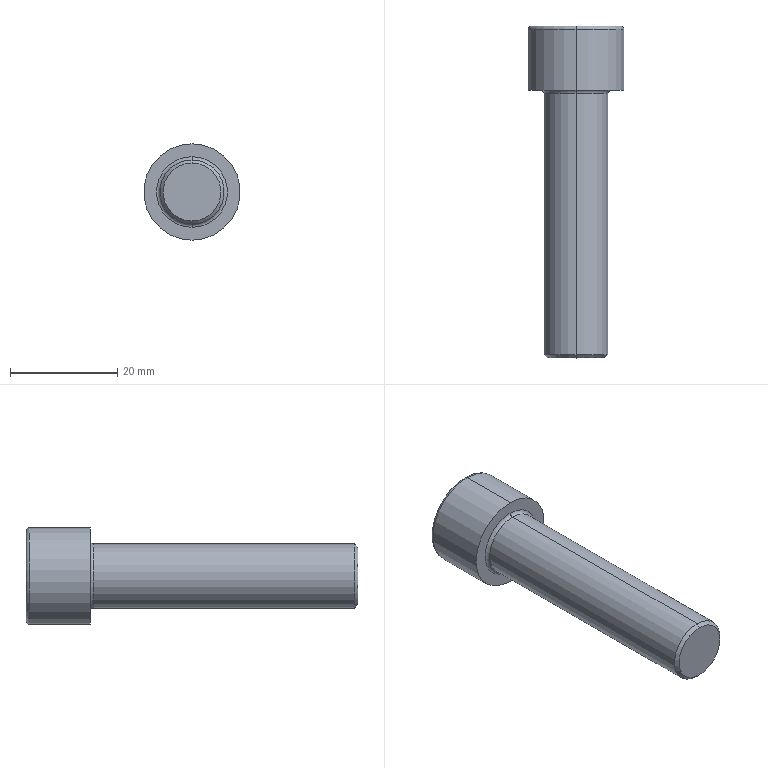Part | STEP file | 1 solid | 20 faces | box 18 x 62 x 18 mm | volume 8181 mm3 | plane 10 | torus 4 | cylinder 4 | cone 2 | commonest cylinder face diameters 12 x2 18 x2
STEP:
#1=CARTESIAN_POINT('',(0.,-50.,-5.4));
#2=VERTEX_POINT('',#1);
#3=CARTESIAN_POINT('',(0.,-50.,5.4));
#4=VERTEX_POINT('',#3);
#5=CARTESIAN_POINT('',(0.,-50.,0.));
#6=DIRECTION('',(0.,-1.,0.));
#7=DIRECTION('',(0.,0.,-1.));
#8=AXIS2_PLACEMENT_3D('',#5,#6,#7);
#9=CIRCLE('',#8,5.4);
#10=EDGE_CURVE('',#2,#4,#9,.T.);
#11=ORIENTED_EDGE('',*,*,#10,.F.);
#12=CARTESIAN_POINT('',(0.,-49.4,-6.));
#13=VERTEX_POINT('',#12);
#14=CARTESIAN_POINT('',(0.,-50.,-5.4));
#15=DIRECTION('',(0.,0.7071,-0.7071));
#16=VECTOR('',#15,1000.);
#17=LINE('',#14,#16);
#18=EDGE_CURVE('',#2,#13,#17,.T.);
#19=ORIENTED_EDGE('',*,*,#18,.T.);
#20=CARTESIAN_POINT('',(0.,-49.4,6.));
#21=VERTEX_POINT('',#20);
#22=CARTESIAN_POINT('',(0.,-49.4,0.));
#23=DIRECTION('',(0.,1.,0.));
#24=DIRECTION('',(0.,0.,-1.));
#25=AXIS2_PLACEMENT_3D('',#22,#23,#24);
#26=CIRCLE('',#25,6.);
#27=EDGE_CURVE('',#21,#13,#26,.T.);
#28=ORIENTED_EDGE('',*,*,#27,.F.);
#29=CARTESIAN_POINT('',(0.,-50.,5.4));
#30=DIRECTION('',(0.,0.7071,0.7071));
#31=VECTOR('',#30,1000.);
#32=LINE('',#29,#31);
#33=EDGE_CURVE('',#4,#21,#32,.T.);
#34=ORIENTED_EDGE('',*,*,#33,.F.);
#35=EDGE_LOOP('',(#11,#19,#28,#34));
#36=FACE_OUTER_BOUND('',#35,.T.);
#37=CARTESIAN_POINT('',(0.,-50.,0.));
#38=DIRECTION('',(0.,1.,0.));
#39=DIRECTION('',(0.,0.,1.));
#40=AXIS2_PLACEMENT_3D('',#37,#38,#39);
#41=CONICAL_SURFACE('',#40,5.4,0.7854);
#42=ADVANCED_FACE('',(#36),#41,.T.);
#43=CARTESIAN_POINT('',(0.,11.4,-9.));
#44=VERTEX_POINT('',#43);
#45=CARTESIAN_POINT('',(0.,11.4,9.));
#46=VERTEX_POINT('',#45);
#47=CARTESIAN_POINT('',(0.,11.4,0.));
#48=DIRECTION('',(0.,-1.,0.));
#49=DIRECTION('',(0.,0.,1.));
#50=AXIS2_PLACEMENT_3D('',#47,#48,#49);
#51=CIRCLE('',#50,9.);
#52=EDGE_CURVE('',#44,#46,#51,.T.);
#53=ORIENTED_EDGE('',*,*,#52,.F.);
#54=CARTESIAN_POINT('',(0.,12.,-8.4));
#55=VERTEX_POINT('',#54);
#56=CARTESIAN_POINT('',(0.,11.4,-8.4));
#57=DIRECTION('',(1.,0.,0.));
#58=DIRECTION('',(0.,0.,-1.));
#59=AXIS2_PLACEMENT_3D('',#56,#57,#58);
#60=CIRCLE('',#59,0.6);
#61=EDGE_CURVE('',#44,#55,#60,.T.);
#62=ORIENTED_EDGE('',*,*,#61,.T.);
#63=CARTESIAN_POINT('',(0.,12.,8.4));
#64=VERTEX_POINT('',#63);
#65=CARTESIAN_POINT('',(0.,12.,0.));
#66=DIRECTION('',(0.,1.,0.));
#67=DIRECTION('',(0.,0.,1.));
#68=AXIS2_PLACEMENT_3D('',#65,#66,#67);
#69=CIRCLE('',#68,8.4);
#70=EDGE_CURVE('',#64,#55,#69,.T.);
#71=ORIENTED_EDGE('',*,*,#70,.F.);
#72=CARTESIAN_POINT('',(0.,11.4,8.4));
#73=DIRECTION('',(-1.,0.,0.));
#74=DIRECTION('',(0.,0.,1.));
#75=AXIS2_PLACEMENT_3D('',#72,#73,#74);
#76=CIRCLE('',#75,0.6);
#77=EDGE_CURVE('',#46,#64,#76,.T.);
#78=ORIENTED_EDGE('',*,*,#77,.F.);
#79=EDGE_LOOP('',(#53,#62,#71,#78));
#80=FACE_OUTER_BOUND('',#79,.T.);
#81=CARTESIAN_POINT('',(0.,11.4,0.));
#82=DIRECTION('',(0.,1.,0.));
#83=DIRECTION('',(0.,0.,1.));
#84=AXIS2_PLACEMENT_3D('',#81,#82,#83);
#85=TOROIDAL_SURFACE('',#84,8.4,0.6);
#86=ADVANCED_FACE('',(#80),#85,.T.);
#87=CARTESIAN_POINT('',(0.,-0.6,6.));
#88=VERTEX_POINT('',#87);
#89=CARTESIAN_POINT('',(0.,-0.6,-6.));
#90=VERTEX_POINT('',#89);
#91=CARTESIAN_POINT('',(0.,-0.6,0.));
#92=DIRECTION('',(0.,-1.,0.));
#93=DIRECTION('',(0.,0.,-1.));
#94=AXIS2_PLACEMENT_3D('',#91,#92,#93);
#95=CIRCLE('',#94,6.);
#96=EDGE_CURVE('',#88,#90,#95,.T.);
#97=ORIENTED_EDGE('',*,*,#96,.F.);
#98=CARTESIAN_POINT('',(0.,0.,6.6));
#99=VERTEX_POINT('',#98);
#100=CARTESIAN_POINT('',(0.,-0.6,6.6));
#101=DIRECTION('',(1.,0.,0.));
#102=DIRECTION('',(0.,0.,-1.));
#103=AXIS2_PLACEMENT_3D('',#100,#101,#102);
#104=CIRCLE('',#103,0.6);
#105=EDGE_CURVE('',#88,#99,#104,.T.);
#106=ORIENTED_EDGE('',*,*,#105,.T.);
#107=CARTESIAN_POINT('',(0.,0.,-6.6));
#108=VERTEX_POINT('',#107);
#109=CARTESIAN_POINT('',(0.,0.,0.));
#110=DIRECTION('',(0.,1.,0.));
#111=DIRECTION('',(0.,0.,-1.));
#112=AXIS2_PLACEMENT_3D('',#109,#110,#111);
#113=CIRCLE('',#112,6.6);
#114=EDGE_CURVE('',#108,#99,#113,.T.);
#115=ORIENTED_EDGE('',*,*,#114,.F.);
#116=CARTESIAN_POINT('',(0.,-0.6,-6.6));
#117=DIRECTION('',(-1.,0.,0.));
#118=DIRECTION('',(0.,0.,1.));
#119=AXIS2_PLACEMENT_3D('',#116,#117,#118);
#120=CIRCLE('',#119,0.6);
#121=EDGE_CURVE('',#90,#108,#120,.T.);
#122=ORIENTED_EDGE('',*,*,#121,.F.);
#123=EDGE_LOOP('',(#97,#106,#115,#122));
#124=FACE_OUTER_BOUND('',#123,.T.);
#125=CARTESIAN_POINT('',(0.,-0.6,0.));
#126=DIRECTION('',(0.,-1.,0.));
#127=DIRECTION('',(0.,0.,-1.));
#128=AXIS2_PLACEMENT_3D('',#125,#126,#127);
#129=TOROIDAL_SURFACE('',#128,6.6,0.6);
#130=ADVANCED_FACE('',(#124),#129,.F.);
#131=CARTESIAN_POINT('',(0.,-0.6,0.));
#132=DIRECTION('',(0.,-1.,0.));
#133=DIRECTION('',(0.,0.,-1.));
#134=AXIS2_PLACEMENT_3D('',#131,#132,#133);
#135=CIRCLE('',#134,6.);
#136=EDGE_CURVE('',#90,#88,#135,.T.);
#137=ORIENTED_EDGE('',*,*,#136,.T.);
#138=CARTESIAN_POINT('',(0.,0.,6.));
#139=DIRECTION('',(0.,-1.,0.));
#140=VECTOR('',#139,1000.);
#141=LINE('',#138,#140);
#142=EDGE_CURVE('',#88,#21,#141,.T.);
#143=ORIENTED_EDGE('',*,*,#142,.T.);
#144=ORIENTED_EDGE('',*,*,#27,.T.);
#145=CARTESIAN_POINT('',(0.,0.,-6.));
#146=DIRECTION('',(0.,-1.,0.));
#147=VECTOR('',#146,1000.);
#148=LINE('',#145,#147);
#149=EDGE_CURVE('',#90,#13,#148,.T.);
#150=ORIENTED_EDGE('',*,*,#149,.F.);
#151=EDGE_LOOP('',(#137,#143,#144,#150));
#152=FACE_OUTER_BOUND('',#151,.T.);
#153=CARTESIAN_POINT('',(0.,0.,0.));
#154=DIRECTION('',(0.,-1.,0.));
#155=DIRECTION('',(0.,0.,-1.));
#156=AXIS2_PLACEMENT_3D('',#153,#154,#155);
#157=CYLINDRICAL_SURFACE('',#156,6.);
#158=ADVANCED_FACE('',(#152),#157,.T.);
#159=ORIENTED_EDGE('',*,*,#52,.T.);
#160=CARTESIAN_POINT('',(0.,0.,9.));
#161=VERTEX_POINT('',#160);
#162=CARTESIAN_POINT('',(0.,0.,9.));
#163=DIRECTION('',(0.,-1.,0.));
#164=VECTOR('',#163,1000.);
#165=LINE('',#162,#164);
#166=EDGE_CURVE('',#46,#161,#165,.T.);
#167=ORIENTED_EDGE('',*,*,#166,.T.);
#168=CARTESIAN_POINT('',(0.,0.,-9.));
#169=VERTEX_POINT('',#168);
#170=CARTESIAN_POINT('',(0.,0.,0.));
#171=DIRECTION('',(0.,-1.,0.));
#172=DIRECTION('',(0.,0.,-1.));
#173=AXIS2_PLACEMENT_3D('',#170,#171,#172);
#174=CIRCLE('',#173,9.);
#175=EDGE_CURVE('',#169,#161,#174,.T.);
#176=ORIENTED_EDGE('',*,*,#175,.F.);
#177=CARTESIAN_POINT('',(0.,0.,-9.));
#178=DIRECTION('',(0.,-1.,0.));
#179=VECTOR('',#178,1000.);
#180=LINE('',#177,#179);
#181=EDGE_CURVE('',#44,#169,#180,.T.);
#182=ORIENTED_EDGE('',*,*,#181,.F.);
#183=EDGE_LOOP('',(#159,#167,#176,#182));
#184=FACE_OUTER_BOUND('',#183,.T.);
#185=CARTESIAN_POINT('',(0.,0.,0.));
#186=DIRECTION('',(0.,-1.,0.));
#187=DIRECTION('',(0.,0.,-1.));
#188=AXIS2_PLACEMENT_3D('',#185,#186,#187);
#189=CYLINDRICAL_SURFACE('',#188,9.);
#190=ADVANCED_FACE('',(#184),#189,.T.);
#191=ORIENTED_EDGE('',*,*,#70,.T.);
#192=CARTESIAN_POINT('',(0.,12.,0.));
#193=DIRECTION('',(0.,1.,0.));
#194=DIRECTION('',(0.,0.,1.));
#195=AXIS2_PLACEMENT_3D('',#192,#193,#194);
#196=CIRCLE('',#195,8.4);
#197=EDGE_CURVE('',#55,#64,#196,.T.);
#198=ORIENTED_EDGE('',*,*,#197,.T.);
#199=EDGE_LOOP('',(#191,#198));
#200=FACE_OUTER_BOUND('',#199,.T.);
#201=CARTESIAN_POINT('',(0.,12.,-5.774));
#202=VERTEX_POINT('',#201);
#203=CARTESIAN_POINT('',(-5.,12.,-2.887));
#204=VERTEX_POINT('',#203);
#205=CARTESIAN_POINT('',(0.,12.,-5.774));
#206=DIRECTION('',(-0.866,0.,0.5));
#207=VECTOR('',#206,1000.);
#208=LINE('',#205,#207);
#209=EDGE_CURVE('',#202,#204,#208,.T.);
#210=ORIENTED_EDGE('',*,*,#209,.F.);
#211=CARTESIAN_POINT('',(5.,12.,-2.887));
#212=VERTEX_POINT('',#211);
#213=CARTESIAN_POINT('',(5.,12.,-2.887));
#214=DIRECTION('',(-0.866,0.,-0.5));
#215=VECTOR('',#214,1000.);
#216=LINE('',#213,#215);
#217=EDGE_CURVE('',#212,#202,#216,.T.);
#218=ORIENTED_EDGE('',*,*,#217,.F.);
#219=CARTESIAN_POINT('',(5.,12.,2.887));
#220=VERTEX_POINT('',#219);
#221=CARTESIAN_POINT('',(5.,12.,2.887));
#222=DIRECTION('',(0.,0.,-1.));
#223=VECTOR('',#222,1000.);
#224=LINE('',#221,#223);
#225=EDGE_CURVE('',#220,#212,#224,.T.);
#226=ORIENTED_EDGE('',*,*,#225,.F.);
#227=CARTESIAN_POINT('',(0.,12.,5.774));
#228=VERTEX_POINT('',#227);
#229=CARTESIAN_POINT('',(0.,12.,5.774));
#230=DIRECTION('',(0.866,0.,-0.5));
#231=VECTOR('',#230,1000.);
#232=LINE('',#229,#231);
#233=EDGE_CURVE('',#228,#220,#232,.T.);
#234=ORIENTED_EDGE('',*,*,#233,.F.);
#235=CARTESIAN_POINT('',(-5.,12.,2.887));
#236=VERTEX_POINT('',#235);
#237=CARTESIAN_POINT('',(-5.,12.,2.887));
#238=DIRECTION('',(0.866,0.,0.5));
#239=VECTOR('',#238,1000.);
#240=LINE('',#237,#239);
#241=EDGE_CURVE('',#236,#228,#240,.T.);
#242=ORIENTED_EDGE('',*,*,#241,.F.);
#243=CARTESIAN_POINT('',(-5.,12.,-2.887));
#244=DIRECTION('',(0.,0.,1.));
#245=VECTOR('',#244,1000.);
#246=LINE('',#243,#245);
#247=EDGE_CURVE('',#204,#236,#246,.T.);
#248=ORIENTED_EDGE('',*,*,#247,.F.);
#249=EDGE_LOOP('',(#210,#218,#226,#234,#242,#248));
#250=FACE_BOUND('',#249,.T.);
#251=CARTESIAN_POINT('',(0.,12.,0.));
#252=DIRECTION('',(0.,1.,0.));
#253=DIRECTION('',(0.,0.,1.));
#254=AXIS2_PLACEMENT_3D('',#251,#252,#253);
#255=PLANE('',#254);
#256=ADVANCED_FACE('',(#200,#250),#255,.T.);
#257=ORIENTED_EDGE('',*,*,#166,.F.);
#258=CARTESIAN_POINT('',(0.,11.4,0.));
#259=DIRECTION('',(0.,-1.,0.));
#260=DIRECTION('',(0.,0.,1.));
#261=AXIS2_PLACEMENT_3D('',#258,#259,#260);
#262=CIRCLE('',#261,9.);
#263=EDGE_CURVE('',#46,#44,#262,.T.);
#264=ORIENTED_EDGE('',*,*,#263,.T.);
#265=ORIENTED_EDGE('',*,*,#181,.T.);
#266=CARTESIAN_POINT('',(0.,0.,0.));
#267=DIRECTION('',(0.,-1.,0.));
#268=DIRECTION('',(0.,0.,-1.));
#269=AXIS2_PLACEMENT_3D('',#266,#267,#268);
#270=CIRCLE('',#269,9.);
#271=EDGE_CURVE('',#161,#169,#270,.T.);
#272=ORIENTED_EDGE('',*,*,#271,.F.);
#273=EDGE_LOOP('',(#257,#264,#265,#272));
#274=FACE_OUTER_BOUND('',#273,.T.);
#275=CARTESIAN_POINT('',(0.,0.,0.));
#276=DIRECTION('',(0.,-1.,0.));
#277=DIRECTION('',(0.,0.,-1.));
#278=AXIS2_PLACEMENT_3D('',#275,#276,#277);
#279=CYLINDRICAL_SURFACE('',#278,9.);
#280=ADVANCED_FACE('',(#274),#279,.T.);
#281=ORIENTED_EDGE('',*,*,#114,.T.);
#282=CARTESIAN_POINT('',(0.,0.,0.));
#283=DIRECTION('',(0.,1.,0.));
#284=DIRECTION('',(0.,0.,-1.));
#285=AXIS2_PLACEMENT_3D('',#282,#283,#284);
#286=CIRCLE('',#285,6.6);
#287=EDGE_CURVE('',#99,#108,#286,.T.);
#288=ORIENTED_EDGE('',*,*,#287,.T.);
#289=EDGE_LOOP('',(#281,#288));
#290=FACE_BOUND('',#289,.T.);
#291=ORIENTED_EDGE('',*,*,#175,.T.);
#292=ORIENTED_EDGE('',*,*,#271,.T.);
#293=EDGE_LOOP('',(#291,#292));
#294=FACE_OUTER_BOUND('',#293,.T.);
#295=CARTESIAN_POINT('',(9.,0.,0.));
#296=DIRECTION('',(0.,-1.,0.));
#297=DIRECTION('',(0.,0.,-1.));
#298=AXIS2_PLACEMENT_3D('',#295,#296,#297);
#299=PLANE('',#298);
#300=ADVANCED_FACE('',(#290,#294),#299,.T.);
#301=ORIENTED_EDGE('',*,*,#142,.F.);
#302=ORIENTED_EDGE('',*,*,#96,.T.);
#303=ORIENTED_EDGE('',*,*,#149,.T.);
#304=CARTESIAN_POINT('',(0.,-49.4,0.));
#305=DIRECTION('',(0.,1.,0.));
#306=DIRECTION('',(0.,0.,-1.));
#307=AXIS2_PLACEMENT_3D('',#304,#305,#306);
#308=CIRCLE('',#307,6.);
#309=EDGE_CURVE('',#13,#21,#308,.T.);
#310=ORIENTED_EDGE('',*,*,#309,.T.);
#311=EDGE_LOOP('',(#301,#302,#303,#310));
#312=FACE_OUTER_BOUND('',#311,.T.);
#313=CARTESIAN_POINT('',(0.,0.,0.));
#314=DIRECTION('',(0.,-1.,0.));
#315=DIRECTION('',(0.,0.,-1.));
#316=AXIS2_PLACEMENT_3D('',#313,#314,#315);
#317=CYLINDRICAL_SURFACE('',#316,6.);
#318=ADVANCED_FACE('',(#312),#317,.T.);
#319=CARTESIAN_POINT('',(0.,-50.,0.));
#320=DIRECTION('',(0.,-1.,0.));
#321=DIRECTION('',(0.,0.,-1.));
#322=AXIS2_PLACEMENT_3D('',#319,#320,#321);
#323=CIRCLE('',#322,5.4);
#324=EDGE_CURVE('',#4,#2,#323,.T.);
#325=ORIENTED_EDGE('',*,*,#324,.T.);
#326=ORIENTED_EDGE('',*,*,#10,.T.);
#327=EDGE_LOOP('',(#325,#326));
#328=FACE_OUTER_BOUND('',#327,.T.);
#329=CARTESIAN_POINT('',(6.,-50.,0.));
#330=DIRECTION('',(0.,-1.,0.));
#331=DIRECTION('',(0.,0.,-1.));
#332=AXIS2_PLACEMENT_3D('',#329,#330,#331);
#333=PLANE('',#332);
#334=ADVANCED_FACE('',(#328),#333,.T.);
#335=ORIENTED_EDGE('',*,*,#209,.T.);
#336=CARTESIAN_POINT('',(-5.,6.,-2.887));
#337=VERTEX_POINT('',#336);
#338=CARTESIAN_POINT('',(-5.,6.,-2.887));
#339=DIRECTION('',(0.,1.,0.));
#340=VECTOR('',#339,1000.);
#341=LINE('',#338,#340);
#342=EDGE_CURVE('',#337,#204,#341,.T.);
#343=ORIENTED_EDGE('',*,*,#342,.F.);
#344=CARTESIAN_POINT('',(0.,6.,-5.774));
#345=VERTEX_POINT('',#344);
#346=CARTESIAN_POINT('',(0.,6.,-5.774));
#347=DIRECTION('',(-0.866,0.,0.5));
#348=VECTOR('',#347,1000.);
#349=LINE('',#346,#348);
#350=EDGE_CURVE('',#345,#337,#349,.T.);
#351=ORIENTED_EDGE('',*,*,#350,.F.);
#352=CARTESIAN_POINT('',(0.,6.,-5.774));
#353=DIRECTION('',(0.,1.,0.));
#354=VECTOR('',#353,1000.);
#355=LINE('',#352,#354);
#356=EDGE_CURVE('',#345,#202,#355,.T.);
#357=ORIENTED_EDGE('',*,*,#356,.T.);
#358=EDGE_LOOP('',(#335,#343,#351,#357));
#359=FACE_OUTER_BOUND('',#358,.T.);
#360=CARTESIAN_POINT('',(0.,6.,-5.774));
#361=DIRECTION('',(-0.5,0.,-0.866));
#362=DIRECTION('',(-0.866,0.,0.5));
#363=AXIS2_PLACEMENT_3D('',#360,#361,#362);
#364=PLANE('',#363);
#365=ADVANCED_FACE('',(#359),#364,.F.);
#366=ORIENTED_EDGE('',*,*,#217,.T.);
#367=ORIENTED_EDGE('',*,*,#356,.F.);
#368=CARTESIAN_POINT('',(5.,6.,-2.887));
#369=VERTEX_POINT('',#368);
#370=CARTESIAN_POINT('',(5.,6.,-2.887));
#371=DIRECTION('',(-0.866,0.,-0.5));
#372=VECTOR('',#371,1000.);
#373=LINE('',#370,#372);
#374=EDGE_CURVE('',#369,#345,#373,.T.);
#375=ORIENTED_EDGE('',*,*,#374,.F.);
#376=CARTESIAN_POINT('',(5.,6.,-2.887));
#377=DIRECTION('',(0.,1.,0.));
#378=VECTOR('',#377,1000.);
#379=LINE('',#376,#378);
#380=EDGE_CURVE('',#369,#212,#379,.T.);
#381=ORIENTED_EDGE('',*,*,#380,.T.);
#382=EDGE_LOOP('',(#366,#367,#375,#381));
#383=FACE_OUTER_BOUND('',#382,.T.);
#384=CARTESIAN_POINT('',(5.,6.,-2.887));
#385=DIRECTION('',(0.5,0.,-0.866));
#386=DIRECTION('',(-0.866,0.,-0.5));
#387=AXIS2_PLACEMENT_3D('',#384,#385,#386);
#388=PLANE('',#387);
#389=ADVANCED_FACE('',(#383),#388,.F.);
#390=ORIENTED_EDGE('',*,*,#225,.T.);
#391=ORIENTED_EDGE('',*,*,#380,.F.);
#392=CARTESIAN_POINT('',(5.,6.,2.887));
#393=VERTEX_POINT('',#392);
#394=CARTESIAN_POINT('',(5.,6.,2.887));
#395=DIRECTION('',(0.,0.,-1.));
#396=VECTOR('',#395,1000.);
#397=LINE('',#394,#396);
#398=EDGE_CURVE('',#393,#369,#397,.T.);
#399=ORIENTED_EDGE('',*,*,#398,.F.);
#400=CARTESIAN_POINT('',(5.,6.,2.887));
#401=DIRECTION('',(0.,1.,0.));
#402=VECTOR('',#401,1000.);
#403=LINE('',#400,#402);
#404=EDGE_CURVE('',#393,#220,#403,.T.);
#405=ORIENTED_EDGE('',*,*,#404,.T.);
#406=EDGE_LOOP('',(#390,#391,#399,#405));
#407=FACE_OUTER_BOUND('',#406,.T.);
#408=CARTESIAN_POINT('',(5.,6.,2.887));
#409=DIRECTION('',(1.,0.,0.));
#410=DIRECTION('',(0.,0.,-1.));
#411=AXIS2_PLACEMENT_3D('',#408,#409,#410);
#412=PLANE('',#411);
#413=ADVANCED_FACE('',(#407),#412,.F.);
#414=ORIENTED_EDGE('',*,*,#233,.T.);
#415=ORIENTED_EDGE('',*,*,#404,.F.);
#416=CARTESIAN_POINT('',(0.,6.,5.774));
#417=VERTEX_POINT('',#416);
#418=CARTESIAN_POINT('',(0.,6.,5.774));
#419=DIRECTION('',(0.866,0.,-0.5));
#420=VECTOR('',#419,1000.);
#421=LINE('',#418,#420);
#422=EDGE_CURVE('',#417,#393,#421,.T.);
#423=ORIENTED_EDGE('',*,*,#422,.F.);
#424=CARTESIAN_POINT('',(0.,6.,5.774));
#425=DIRECTION('',(0.,1.,0.));
#426=VECTOR('',#425,1000.);
#427=LINE('',#424,#426);
#428=EDGE_CURVE('',#417,#228,#427,.T.);
#429=ORIENTED_EDGE('',*,*,#428,.T.);
#430=EDGE_LOOP('',(#414,#415,#423,#429));
#431=FACE_OUTER_BOUND('',#430,.T.);
#432=CARTESIAN_POINT('',(0.,6.,5.774));
#433=DIRECTION('',(0.5,0.,0.866));
#434=DIRECTION('',(0.866,0.,-0.5));
#435=AXIS2_PLACEMENT_3D('',#432,#433,#434);
#436=PLANE('',#435);
#437=ADVANCED_FACE('',(#431),#436,.F.);
#438=ORIENTED_EDGE('',*,*,#241,.T.);
#439=ORIENTED_EDGE('',*,*,#428,.F.);
#440=CARTESIAN_POINT('',(-5.,6.,2.887));
#441=VERTEX_POINT('',#440);
#442=CARTESIAN_POINT('',(-5.,6.,2.887));
#443=DIRECTION('',(0.866,0.,0.5));
#444=VECTOR('',#443,1000.);
#445=LINE('',#442,#444);
#446=EDGE_CURVE('',#441,#417,#445,.T.);
#447=ORIENTED_EDGE('',*,*,#446,.F.);
#448=CARTESIAN_POINT('',(-5.,6.,2.887));
#449=DIRECTION('',(0.,1.,0.));
#450=VECTOR('',#449,1000.);
#451=LINE('',#448,#450);
#452=EDGE_CURVE('',#441,#236,#451,.T.);
#453=ORIENTED_EDGE('',*,*,#452,.T.);
#454=EDGE_LOOP('',(#438,#439,#447,#453));
#455=FACE_OUTER_BOUND('',#454,.T.);
#456=CARTESIAN_POINT('',(-5.,6.,2.887));
#457=DIRECTION('',(-0.5,0.,0.866));
#458=DIRECTION('',(0.866,0.,0.5));
#459=AXIS2_PLACEMENT_3D('',#456,#457,#458);
#460=PLANE('',#459);
#461=ADVANCED_FACE('',(#455),#460,.F.);
#462=ORIENTED_EDGE('',*,*,#247,.T.);
#463=ORIENTED_EDGE('',*,*,#452,.F.);
#464=CARTESIAN_POINT('',(-5.,6.,-2.887));
#465=DIRECTION('',(0.,0.,1.));
#466=VECTOR('',#465,1000.);
#467=LINE('',#464,#466);
#468=EDGE_CURVE('',#337,#441,#467,.T.);
#469=ORIENTED_EDGE('',*,*,#468,.F.);
#470=ORIENTED_EDGE('',*,*,#342,.T.);
#471=EDGE_LOOP('',(#462,#463,#469,#470));
#472=FACE_OUTER_BOUND('',#471,.T.);
#473=CARTESIAN_POINT('',(-5.,6.,-2.887));
#474=DIRECTION('',(-1.,0.,0.));
#475=DIRECTION('',(0.,0.,1.));
#476=AXIS2_PLACEMENT_3D('',#473,#474,#475);
#477=PLANE('',#476);
#478=ADVANCED_FACE('',(#472),#477,.F.);
#479=ORIENTED_EDGE('',*,*,#350,.T.);
#480=ORIENTED_EDGE('',*,*,#468,.T.);
#481=ORIENTED_EDGE('',*,*,#446,.T.);
#482=ORIENTED_EDGE('',*,*,#422,.T.);
#483=ORIENTED_EDGE('',*,*,#398,.T.);
#484=ORIENTED_EDGE('',*,*,#374,.T.);
#485=EDGE_LOOP('',(#479,#480,#481,#482,#483,#484));
#486=FACE_OUTER_BOUND('',#485,.T.);
#487=CARTESIAN_POINT('',(0.,6.,0.));
#488=DIRECTION('',(0.,1.,0.));
#489=DIRECTION('',(0.,0.,1.));
#490=AXIS2_PLACEMENT_3D('',#487,#488,#489);
#491=PLANE('',#490);
#492=ADVANCED_FACE('',(#486),#491,.T.);
#493=ORIENTED_EDGE('',*,*,#105,.F.);
#494=ORIENTED_EDGE('',*,*,#136,.F.);
#495=ORIENTED_EDGE('',*,*,#121,.T.);
#496=ORIENTED_EDGE('',*,*,#287,.F.);
#497=EDGE_LOOP('',(#493,#494,#495,#496));
#498=FACE_OUTER_BOUND('',#497,.T.);
#499=CARTESIAN_POINT('',(0.,-0.6,0.));
#500=DIRECTION('',(0.,-1.,0.));
#501=DIRECTION('',(0.,0.,-1.));
#502=AXIS2_PLACEMENT_3D('',#499,#500,#501);
#503=TOROIDAL_SURFACE('',#502,6.6,0.6);
#504=ADVANCED_FACE('',(#498),#503,.F.);
#505=ORIENTED_EDGE('',*,*,#61,.F.);
#506=ORIENTED_EDGE('',*,*,#263,.F.);
#507=ORIENTED_EDGE('',*,*,#77,.T.);
#508=ORIENTED_EDGE('',*,*,#197,.F.);
#509=EDGE_LOOP('',(#505,#506,#507,#508));
#510=FACE_OUTER_BOUND('',#509,.T.);
#511=CARTESIAN_POINT('',(0.,11.4,0.));
#512=DIRECTION('',(0.,1.,0.));
#513=DIRECTION('',(0.,0.,1.));
#514=AXIS2_PLACEMENT_3D('',#511,#512,#513);
#515=TOROIDAL_SURFACE('',#514,8.4,0.6);
#516=ADVANCED_FACE('',(#510),#515,.T.);
#517=ORIENTED_EDGE('',*,*,#18,.F.);
#518=ORIENTED_EDGE('',*,*,#324,.F.);
#519=ORIENTED_EDGE('',*,*,#33,.T.);
#520=ORIENTED_EDGE('',*,*,#309,.F.);
#521=EDGE_LOOP('',(#517,#518,#519,#520));
#522=FACE_OUTER_BOUND('',#521,.T.);
#523=CARTESIAN_POINT('',(0.,-50.,0.));
#524=DIRECTION('',(0.,1.,0.));
#525=DIRECTION('',(0.,0.,1.));
#526=AXIS2_PLACEMENT_3D('',#523,#524,#525);
#527=CONICAL_SURFACE('',#526,5.4,0.7854);
#528=ADVANCED_FACE('',(#522),#527,.T.);
#529=CLOSED_SHELL('',(#42,#86,#130,#158,#190,#256,#280,#300,#318,#334,#365,#389,#413,#437,#461,#478,#492,#504,#516,#528));
#530=MANIFOLD_SOLID_BREP('',#529);
#531=CARTESIAN_POINT('',(0.,0.,0.));
#532=DIRECTION('',(0.,0.,1.));
#533=DIRECTION('',(1.,0.,0.));
#534=AXIS2_PLACEMENT_3D('',#531,#532,#533);
#535=(LENGTH_UNIT()NAMED_UNIT(*)SI_UNIT(.MILLI.,.METRE.));
#536=UNCERTAINTY_MEASURE_WITH_UNIT(LENGTH_MEASURE(0.00001),#535,'','');
#537=(NAMED_UNIT(*)PLANE_ANGLE_UNIT()SI_UNIT($,.RADIAN.));
#538=(NAMED_UNIT(*)SI_UNIT($,.STERADIAN.)SOLID_ANGLE_UNIT());
#539=(GEOMETRIC_REPRESENTATION_CONTEXT(3)GLOBAL_UNCERTAINTY_ASSIGNED_CONTEXT((#536))GLOBAL_UNIT_ASSIGNED_CONTEXT((#535,#537,#538))REPRESENTATION_CONTEXT('',''));
#540=ADVANCED_BREP_SHAPE_REPRESENTATION('',(#530,#534),#539);